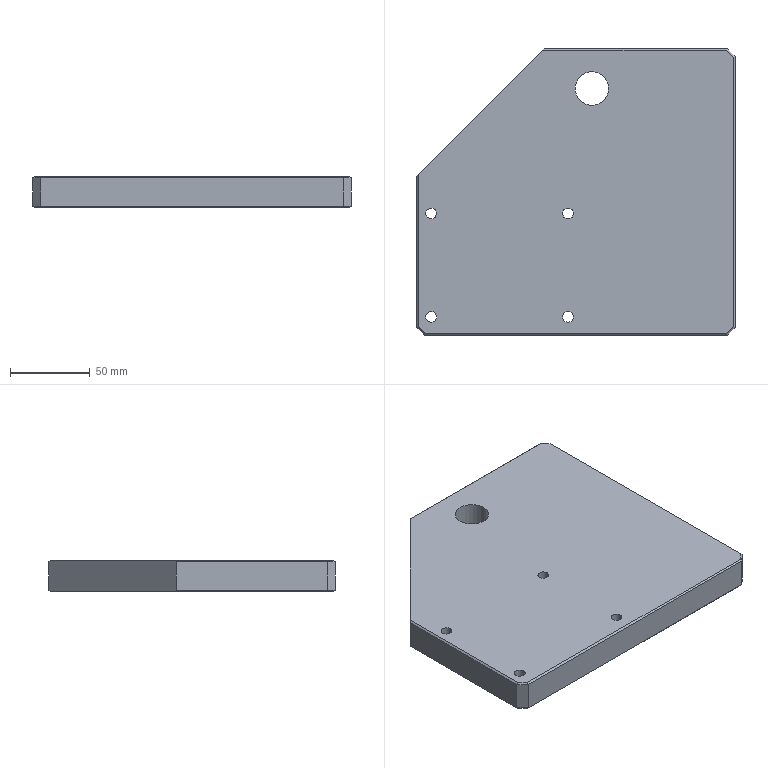Part | STEP file | 1 solid | 34 faces | box 200 x 180 x 20 mm | volume 644827 mm3 | plane 24 | cylinder 10 | commonest cylinder face diameters 6.8 x8 21 x2